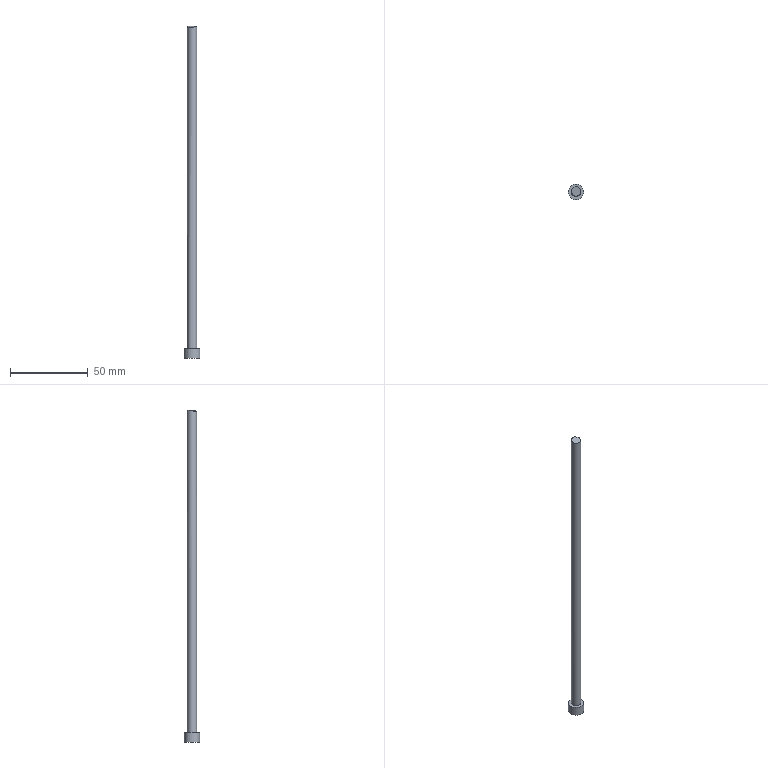Part | NX | features DDZ6.00 2 | 1 solid | 5 faces | box 10 x 10 x 213.511 mm | volume 6325 mm3 | cylinder 2 | plane 2 | sphere 1 | commonest cylinder face diameters 6 x1 10 x1
STEP:
#1=CARTESIAN_POINT('',(-12.41,-34.38,-204.5));
#2=VERTEX_POINT('',#1);
#3=CARTESIAN_POINT('',(-15.41,-34.38,-204.5));
#4=DIRECTION('',(0.,0.,1.));
#5=DIRECTION('',(1.,0.,0.));
#6=AXIS2_PLACEMENT_3D('',#3,#4,#5);
#7=CIRCLE('',#6,3.);
#8=EDGE_CURVE('',#2,#2,#7,.F.);
#9=ORIENTED_EDGE('',*,*,#8,.F.);
#10=EDGE_LOOP('',(#9));
#11=FACE_BOUND('',#10,.T.);
#12=CARTESIAN_POINT('',(-17.537,-36.496,2.209));
#13=VERTEX_POINT('',#12);
#14=CARTESIAN_POINT('',(-15.401,-37.708,2.177));
#15=CARTESIAN_POINT('',(-17.772,-36.725,2.167));
#16=CARTESIAN_POINT('',(-18.731,-34.367,2.411));
#17=CARTESIAN_POINT('',(-17.763,-32.037,2.76));
#18=CARTESIAN_POINT('',(-15.419,-31.052,3.016));
#19=CARTESIAN_POINT('',(-13.049,-32.035,3.026));
#20=CARTESIAN_POINT('',(-12.089,-34.389,2.784));
#21=CARTESIAN_POINT('',(-13.055,-36.723,2.434));
#22=CARTESIAN_POINT('',(-15.401,-37.708,2.177));
#23=CARTESIAN_POINT('',(-17.772,-36.725,2.167));
#24=CARTESIAN_POINT('',(-18.731,-34.367,2.411));
#25=B_SPLINE_CURVE_WITH_KNOTS('',3,(#14,#15,#16,#17,#18,#19,#20,#21,#22,#23,#24),.UNSPECIFIED.,.T.,.F.,(1,1,1,1,1,1,1,1,1,1,1,1,1,1,1),(-0.007067,-0.004712,-0.002356,0.,0.002356,0.004712,0.007067,0.009423,0.01178,0.01413,0.01649,0.01885,0.0212,0.02356,0.02591),.UNSPECIFIED.);
#26=EDGE_CURVE('',#13,#13,#25,.T.);
#27=ORIENTED_EDGE('',*,*,#26,.T.);
#28=EDGE_LOOP('',(#27));
#29=FACE_BOUND('',#28,.T.);
#30=CARTESIAN_POINT('',(-15.41,-34.38,-210.5));
#31=DIRECTION('',(0.,0.,1.));
#32=DIRECTION('',(1.,0.,0.));
#33=AXIS2_PLACEMENT_3D('',#30,#31,#32);
#34=CYLINDRICAL_SURFACE('',#33,3.);
#35=ADVANCED_FACE('',(#11,#29),#34,.T.);
#36=ORIENTED_EDGE('',*,*,#8,.T.);
#37=EDGE_LOOP('',(#36));
#38=FACE_BOUND('',#37,.T.);
#39=CARTESIAN_POINT('',(-10.41,-34.38,-204.5));
#40=VERTEX_POINT('',#39);
#41=CARTESIAN_POINT('',(-15.41,-34.38,-204.5));
#42=DIRECTION('',(0.,0.,-1.));
#43=DIRECTION('',(1.,0.,0.));
#44=AXIS2_PLACEMENT_3D('',#41,#42,#43);
#45=CIRCLE('',#44,5.);
#46=EDGE_CURVE('',#40,#40,#45,.T.);
#47=ORIENTED_EDGE('',*,*,#46,.F.);
#48=EDGE_LOOP('',(#47));
#49=FACE_BOUND('',#48,.T.);
#50=CARTESIAN_POINT('',(-15.41,-34.38,-204.5));
#51=DIRECTION('',(0.,0.,1.));
#52=DIRECTION('',(1.,0.,0.));
#53=AXIS2_PLACEMENT_3D('',#50,#51,#52);
#54=PLANE('',#53);
#55=ADVANCED_FACE('',(#38,#49),#54,.T.);
#56=ORIENTED_EDGE('',*,*,#46,.T.);
#57=EDGE_LOOP('',(#56));
#58=FACE_BOUND('',#57,.T.);
#59=CARTESIAN_POINT('',(-10.41,-34.38,-210.5));
#60=VERTEX_POINT('',#59);
#61=CARTESIAN_POINT('',(-15.41,-34.38,-210.5));
#62=DIRECTION('',(0.,0.,1.));
#63=DIRECTION('',(1.,0.,0.));
#64=AXIS2_PLACEMENT_3D('',#61,#62,#63);
#65=CIRCLE('',#64,5.);
#66=EDGE_CURVE('',#60,#60,#65,.T.);
#67=ORIENTED_EDGE('',*,*,#66,.T.);
#68=EDGE_LOOP('',(#67));
#69=FACE_BOUND('',#68,.T.);
#70=CARTESIAN_POINT('',(-15.41,-34.38,-210.5));
#71=DIRECTION('',(0.,0.,1.));
#72=DIRECTION('',(1.,0.,0.));
#73=AXIS2_PLACEMENT_3D('',#70,#71,#72);
#74=CYLINDRICAL_SURFACE('',#73,5.);
#75=ADVANCED_FACE('',(#58,#69),#74,.T.);
#76=ORIENTED_EDGE('',*,*,#66,.F.);
#77=EDGE_LOOP('',(#76));
#78=FACE_BOUND('',#77,.T.);
#79=CARTESIAN_POINT('',(-15.41,-34.38,-210.5));
#80=DIRECTION('',(0.,0.,-1.));
#81=DIRECTION('',(-1.,0.,0.));
#82=AXIS2_PLACEMENT_3D('',#79,#80,#81);
#83=PLANE('',#82);
#84=ADVANCED_FACE('',(#78),#83,.T.);
#85=ORIENTED_EDGE('',*,*,#26,.F.);
#86=EDGE_LOOP('',(#85));
#87=FACE_BOUND('',#86,.T.);
#88=CARTESIAN_POINT('',(0.,0.,-269.66));
#89=DIRECTION('',(0.,0.,-1.));
#90=DIRECTION('',(1.,0.,0.));
#91=AXIS2_PLACEMENT_3D('',#88,#89,#90);
#92=SPHERICAL_SURFACE('',#91,274.868);
#93=ADVANCED_FACE('',(#87),#92,.T.);
#94=CLOSED_SHELL('',(#35,#55,#75,#84,#93));
#95=MANIFOLD_SOLID_BREP('',#94);
#96=(LENGTH_UNIT()NAMED_UNIT(*)SI_UNIT(.MILLI.,.METRE.));
#97=UNCERTAINTY_MEASURE_WITH_UNIT(LENGTH_MEASURE(0.0508),#96,'','');
#98=(NAMED_UNIT(*)PLANE_ANGLE_UNIT()SI_UNIT($,.RADIAN.));
#99=(NAMED_UNIT(*)SI_UNIT($,.STERADIAN.)SOLID_ANGLE_UNIT());
#100=(GEOMETRIC_REPRESENTATION_CONTEXT(3)GLOBAL_UNCERTAINTY_ASSIGNED_CONTEXT((#97))GLOBAL_UNIT_ASSIGNED_CONTEXT((#96,#98,#99))REPRESENTATION_CONTEXT('',''));
#101=ADVANCED_BREP_SHAPE_REPRESENTATION('',(#95),#100);